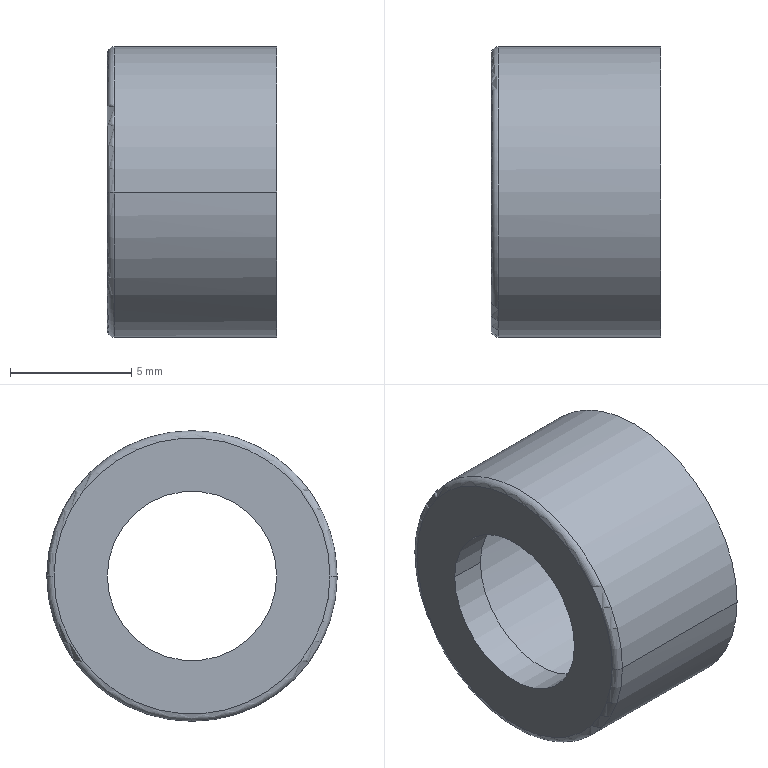Part | STEP file | SHIMOZHOUCHENGWAITAO_6_1_2_3_2_ | 1 solid | 15 faces | box 7 x 12 x 12 mm | volume 297.806 mm3 | cylinder 6 | torus 4 | plane 3 | cone 2 | commonest cylinder face diameters 7 x2 10 x2 12 x2
STEP:
#1=CARTESIAN_POINT('',(0.,0.,0.));
#2=DIRECTION('',(0.,0.,1.));
#3=DIRECTION('',(1.,0.,0.));
#4=AXIS2_PLACEMENT_3D('',#1,#2,#3);
#5=CARTESIAN_POINT('',(0.,-5.7,-0.03809));
#6=VERTEX_POINT('',#5);
#7=CARTESIAN_POINT('',(0.,-5.7,0.));
#8=VERTEX_POINT('',#7);
#9=CARTESIAN_POINT('',(0.,0.,0.));
#10=DIRECTION('',(-1.,0.,0.));
#11=DIRECTION('',(0.,-1.,-0.006683));
#12=AXIS2_PLACEMENT_3D('',#9,#10,#11);
#13=CIRCLE('',#12,5.7);
#14=EDGE_CURVE('',#6,#8,#13,.T.);
#15=ORIENTED_EDGE('',*,*,#14,.F.);
#16=CARTESIAN_POINT('',(0.,5.7,0.));
#17=VERTEX_POINT('',#16);
#18=CARTESIAN_POINT('',(0.,0.,0.));
#19=DIRECTION('',(1.,0.,0.));
#20=DIRECTION('',(0.,-1.,-0.006683));
#21=AXIS2_PLACEMENT_3D('',#18,#19,#20);
#22=CIRCLE('',#21,5.7);
#23=EDGE_CURVE('',#6,#17,#22,.T.);
#24=ORIENTED_EDGE('',*,*,#23,.T.);
#25=CARTESIAN_POINT('',(0.,5.7,0.03809));
#26=VERTEX_POINT('',#25);
#27=CARTESIAN_POINT('',(0.,0.,0.));
#28=DIRECTION('',(-1.,0.,0.));
#29=DIRECTION('',(0.,1.,0.006683));
#30=AXIS2_PLACEMENT_3D('',#27,#28,#29);
#31=CIRCLE('',#30,5.7);
#32=EDGE_CURVE('',#26,#17,#31,.T.);
#33=ORIENTED_EDGE('',*,*,#32,.F.);
#34=CARTESIAN_POINT('',(0.,0.,0.));
#35=DIRECTION('',(1.,0.,0.));
#36=DIRECTION('',(0.,1.,0.006683));
#37=AXIS2_PLACEMENT_3D('',#34,#35,#36);
#38=CIRCLE('',#37,5.7);
#39=EDGE_CURVE('',#26,#8,#38,.T.);
#40=ORIENTED_EDGE('',*,*,#39,.T.);
#41=EDGE_LOOP('',(#15,#24,#33,#40));
#42=FACE_OUTER_BOUND('',#41,.F.);
#43=CARTESIAN_POINT('',(0.,3.5,0.));
#44=VERTEX_POINT('',#43);
#45=CARTESIAN_POINT('',(0.,-3.5,0.));
#46=VERTEX_POINT('',#45);
#47=CARTESIAN_POINT('',(0.,0.,0.));
#48=DIRECTION('',(-1.,0.,0.));
#49=DIRECTION('',(0.,1.,0.));
#50=AXIS2_PLACEMENT_3D('',#47,#48,#49);
#51=CIRCLE('',#50,3.5);
#52=EDGE_CURVE('',#44,#46,#51,.T.);
#53=ORIENTED_EDGE('',*,*,#52,.T.);
#54=CARTESIAN_POINT('',(0.,0.,0.));
#55=DIRECTION('',(-1.,0.,0.));
#56=DIRECTION('',(0.,-1.,0.));
#57=AXIS2_PLACEMENT_3D('',#54,#55,#56);
#58=CIRCLE('',#57,3.5);
#59=EDGE_CURVE('',#46,#44,#58,.T.);
#60=ORIENTED_EDGE('',*,*,#59,.T.);
#61=EDGE_LOOP('',(#53,#60));
#62=FACE_BOUND('',#61,.F.);
#63=CARTESIAN_POINT('',(0.,0.,0.));
#64=DIRECTION('',(1.,0.,0.));
#65=DIRECTION('',(0.,-1.,0.));
#66=AXIS2_PLACEMENT_3D('',#63,#64,#65);
#67=PLANE('',#66);
#68=ADVANCED_FACE('',(#42,#62),#67,.F.);
#69=ORIENTED_EDGE('',*,*,#23,.F.);
#70=ORIENTED_EDGE('',*,*,#14,.T.);
#71=CARTESIAN_POINT('',(0.3,-6.,0.));
#72=VERTEX_POINT('',#71);
#73=CARTESIAN_POINT('',(0.3,-5.7,0.));
#74=DIRECTION('',(0.,0.,1.));
#75=DIRECTION('',(-1.,0.,0.));
#76=AXIS2_PLACEMENT_3D('',#73,#74,#75);
#77=CIRCLE('',#76,0.3);
#78=EDGE_CURVE('',#8,#72,#77,.T.);
#79=ORIENTED_EDGE('',*,*,#78,.T.);
#80=CARTESIAN_POINT('',(0.3,-6.,-0.0401));
#81=VERTEX_POINT('',#80);
#82=CARTESIAN_POINT('',(0.3,0.,0.));
#83=DIRECTION('',(1.,0.,0.));
#84=DIRECTION('',(0.,-1.,0.));
#85=AXIS2_PLACEMENT_3D('',#82,#83,#84);
#86=CIRCLE('',#85,6.);
#87=EDGE_CURVE('',#72,#81,#86,.T.);
#88=ORIENTED_EDGE('',*,*,#87,.T.);
#89=CARTESIAN_POINT('',(0.3,6.,0.));
#90=VERTEX_POINT('',#89);
#91=CARTESIAN_POINT('',(0.3,0.,0.));
#92=DIRECTION('',(1.,0.,0.));
#93=DIRECTION('',(0.,-1.,-0.006683));
#94=AXIS2_PLACEMENT_3D('',#91,#92,#93);
#95=CIRCLE('',#94,6.);
#96=EDGE_CURVE('',#81,#90,#95,.T.);
#97=ORIENTED_EDGE('',*,*,#96,.T.);
#98=CARTESIAN_POINT('',(0.3,5.7,0.));
#99=DIRECTION('',(0.,0.,-1.));
#100=DIRECTION('',(-1.,0.,0.));
#101=AXIS2_PLACEMENT_3D('',#98,#99,#100);
#102=CIRCLE('',#101,0.3);
#103=EDGE_CURVE('',#17,#90,#102,.T.);
#104=ORIENTED_EDGE('',*,*,#103,.F.);
#105=EDGE_LOOP('',(#69,#70,#79,#88,#97,#104));
#106=FACE_OUTER_BOUND('',#105,.F.);
#107=CARTESIAN_POINT('',(0.3,0.,0.));
#108=DIRECTION('',(1.,0.,0.));
#109=DIRECTION('',(0.,1.,0.006683));
#110=AXIS2_PLACEMENT_3D('',#107,#108,#109);
#111=TOROIDAL_SURFACE('',#110,5.7,0.3);
#112=ADVANCED_FACE('',(#106),#111,.T.);
#113=ORIENTED_EDGE('',*,*,#39,.F.);
#114=ORIENTED_EDGE('',*,*,#32,.T.);
#115=ORIENTED_EDGE('',*,*,#103,.T.);
#116=CARTESIAN_POINT('',(0.3,6.,0.0401));
#117=VERTEX_POINT('',#116);
#118=CARTESIAN_POINT('',(0.3,0.,0.));
#119=DIRECTION('',(1.,0.,0.));
#120=DIRECTION('',(0.,1.,0.));
#121=AXIS2_PLACEMENT_3D('',#118,#119,#120);
#122=CIRCLE('',#121,6.);
#123=EDGE_CURVE('',#90,#117,#122,.T.);
#124=ORIENTED_EDGE('',*,*,#123,.T.);
#125=CARTESIAN_POINT('',(0.3,0.,0.));
#126=DIRECTION('',(1.,0.,0.));
#127=DIRECTION('',(0.,1.,0.006683));
#128=AXIS2_PLACEMENT_3D('',#125,#126,#127);
#129=CIRCLE('',#128,6.);
#130=EDGE_CURVE('',#117,#72,#129,.T.);
#131=ORIENTED_EDGE('',*,*,#130,.T.);
#132=ORIENTED_EDGE('',*,*,#78,.F.);
#133=EDGE_LOOP('',(#113,#114,#115,#124,#131,#132));
#134=FACE_OUTER_BOUND('',#133,.F.);
#135=CARTESIAN_POINT('',(0.3,0.,0.));
#136=DIRECTION('',(1.,0.,0.));
#137=DIRECTION('',(0.,-1.,-0.006683));
#138=AXIS2_PLACEMENT_3D('',#135,#136,#137);
#139=TOROIDAL_SURFACE('',#138,5.7,0.3);
#140=ADVANCED_FACE('',(#134),#139,.T.);
#141=ORIENTED_EDGE('',*,*,#130,.F.);
#142=ORIENTED_EDGE('',*,*,#123,.F.);
#143=CARTESIAN_POINT('',(7.,6.,0.));
#144=VERTEX_POINT('',#143);
#145=CARTESIAN_POINT('',(0.3,6.,0.));
#146=DIRECTION('',(1.,0.,0.));
#147=VECTOR('',#146,6.7);
#148=LINE('',#145,#147);
#149=EDGE_CURVE('',#90,#144,#148,.T.);
#150=ORIENTED_EDGE('',*,*,#149,.T.);
#151=CARTESIAN_POINT('',(7.,-6.,0.));
#152=VERTEX_POINT('',#151);
#153=CARTESIAN_POINT('',(7.,0.,0.));
#154=DIRECTION('',(-1.,0.,0.));
#155=DIRECTION('',(0.,-1.,0.));
#156=AXIS2_PLACEMENT_3D('',#153,#154,#155);
#157=CIRCLE('',#156,6.);
#158=EDGE_CURVE('',#152,#144,#157,.T.);
#159=ORIENTED_EDGE('',*,*,#158,.F.);
#160=CARTESIAN_POINT('',(0.3,-6.,0.));
#161=DIRECTION('',(1.,0.,0.));
#162=VECTOR('',#161,6.7);
#163=LINE('',#160,#162);
#164=EDGE_CURVE('',#72,#152,#163,.T.);
#165=ORIENTED_EDGE('',*,*,#164,.F.);
#166=EDGE_LOOP('',(#141,#142,#150,#159,#165));
#167=FACE_OUTER_BOUND('',#166,.F.);
#168=CARTESIAN_POINT('',(0.,0.,0.));
#169=DIRECTION('',(1.,0.,0.));
#170=DIRECTION('',(0.,-1.,0.));
#171=AXIS2_PLACEMENT_3D('',#168,#169,#170);
#172=CYLINDRICAL_SURFACE('',#171,6.);
#173=ADVANCED_FACE('',(#167),#172,.T.);
#174=ORIENTED_EDGE('',*,*,#96,.F.);
#175=ORIENTED_EDGE('',*,*,#87,.F.);
#176=ORIENTED_EDGE('',*,*,#164,.T.);
#177=CARTESIAN_POINT('',(7.,0.,0.));
#178=DIRECTION('',(-1.,0.,0.));
#179=DIRECTION('',(0.,1.,0.));
#180=AXIS2_PLACEMENT_3D('',#177,#178,#179);
#181=CIRCLE('',#180,6.);
#182=EDGE_CURVE('',#144,#152,#181,.T.);
#183=ORIENTED_EDGE('',*,*,#182,.F.);
#184=ORIENTED_EDGE('',*,*,#149,.F.);
#185=EDGE_LOOP('',(#174,#175,#176,#183,#184));
#186=FACE_OUTER_BOUND('',#185,.F.);
#187=CARTESIAN_POINT('',(0.,0.,0.));
#188=DIRECTION('',(1.,0.,0.));
#189=DIRECTION('',(0.,-1.,0.));
#190=AXIS2_PLACEMENT_3D('',#187,#188,#189);
#191=CYLINDRICAL_SURFACE('',#190,6.);
#192=ADVANCED_FACE('',(#186),#191,.T.);
#193=ORIENTED_EDGE('',*,*,#182,.T.);
#194=ORIENTED_EDGE('',*,*,#158,.T.);
#195=EDGE_LOOP('',(#193,#194));
#196=FACE_OUTER_BOUND('',#195,.F.);
#197=CARTESIAN_POINT('',(7.,-5.5,0.));
#198=VERTEX_POINT('',#197);
#199=CARTESIAN_POINT('',(7.,0.,-5.5));
#200=VERTEX_POINT('',#199);
#201=CARTESIAN_POINT('',(7.,0.,0.));
#202=DIRECTION('',(1.,0.,0.));
#203=DIRECTION('',(0.,-1.,0.));
#204=AXIS2_PLACEMENT_3D('',#201,#202,#203);
#205=CIRCLE('',#204,5.5);
#206=EDGE_CURVE('',#198,#200,#205,.T.);
#207=ORIENTED_EDGE('',*,*,#206,.T.);
#208=CARTESIAN_POINT('',(7.,5.5,0.));
#209=VERTEX_POINT('',#208);
#210=CARTESIAN_POINT('',(7.,0.,0.));
#211=DIRECTION('',(1.,0.,0.));
#212=DIRECTION('',(0.,0.,-1.));
#213=AXIS2_PLACEMENT_3D('',#210,#211,#212);
#214=CIRCLE('',#213,5.5);
#215=EDGE_CURVE('',#200,#209,#214,.T.);
#216=ORIENTED_EDGE('',*,*,#215,.T.);
#217=CARTESIAN_POINT('',(7.,0.,5.5));
#218=VERTEX_POINT('',#217);
#219=CARTESIAN_POINT('',(7.,0.,0.));
#220=DIRECTION('',(1.,0.,0.));
#221=DIRECTION('',(0.,1.,0.));
#222=AXIS2_PLACEMENT_3D('',#219,#220,#221);
#223=CIRCLE('',#222,5.5);
#224=EDGE_CURVE('',#209,#218,#223,.T.);
#225=ORIENTED_EDGE('',*,*,#224,.T.);
#226=CARTESIAN_POINT('',(7.,0.,0.));
#227=DIRECTION('',(1.,0.,0.));
#228=DIRECTION('',(0.,0.,1.));
#229=AXIS2_PLACEMENT_3D('',#226,#227,#228);
#230=CIRCLE('',#229,5.5);
#231=EDGE_CURVE('',#218,#198,#230,.T.);
#232=ORIENTED_EDGE('',*,*,#231,.T.);
#233=EDGE_LOOP('',(#207,#216,#225,#232));
#234=FACE_BOUND('',#233,.F.);
#235=CARTESIAN_POINT('',(7.,0.,0.));
#236=DIRECTION('',(1.,0.,0.));
#237=DIRECTION('',(0.,-1.,0.));
#238=AXIS2_PLACEMENT_3D('',#235,#236,#237);
#239=PLANE('',#238);
#240=ADVANCED_FACE('',(#196,#234),#239,.T.);
#241=ORIENTED_EDGE('',*,*,#215,.F.);
#242=ORIENTED_EDGE('',*,*,#206,.F.);
#243=CARTESIAN_POINT('',(6.5,-5.,0.));
#244=VERTEX_POINT('',#243);
#245=CARTESIAN_POINT('',(7.,-5.5,0.));
#246=DIRECTION('',(-0.7071,0.7071,0.));
#247=VECTOR('',#246,0.7071);
#248=LINE('',#245,#247);
#249=EDGE_CURVE('',#198,#244,#248,.T.);
#250=ORIENTED_EDGE('',*,*,#249,.T.);
#251=CARTESIAN_POINT('',(6.5,0.,-5.));
#252=VERTEX_POINT('',#251);
#253=CARTESIAN_POINT('',(6.5,0.,0.));
#254=DIRECTION('',(1.,0.,0.));
#255=DIRECTION('',(0.,-1.,0.));
#256=AXIS2_PLACEMENT_3D('',#253,#254,#255);
#257=CIRCLE('',#256,5.);
#258=EDGE_CURVE('',#244,#252,#257,.T.);
#259=ORIENTED_EDGE('',*,*,#258,.T.);
#260=CARTESIAN_POINT('',(6.5,5.,0.));
#261=VERTEX_POINT('',#260);
#262=CARTESIAN_POINT('',(6.5,0.,0.));
#263=DIRECTION('',(1.,0.,0.));
#264=DIRECTION('',(0.,0.,-1.));
#265=AXIS2_PLACEMENT_3D('',#262,#263,#264);
#266=CIRCLE('',#265,5.);
#267=EDGE_CURVE('',#252,#261,#266,.T.);
#268=ORIENTED_EDGE('',*,*,#267,.T.);
#269=CARTESIAN_POINT('',(7.,5.5,0.));
#270=DIRECTION('',(-0.7071,-0.7071,0.));
#271=VECTOR('',#270,0.7071);
#272=LINE('',#269,#271);
#273=EDGE_CURVE('',#209,#261,#272,.T.);
#274=ORIENTED_EDGE('',*,*,#273,.F.);
#275=EDGE_LOOP('',(#241,#242,#250,#259,#268,#274));
#276=FACE_OUTER_BOUND('',#275,.F.);
#277=CARTESIAN_POINT('',(6.75,0.,0.));
#278=DIRECTION('',(1.,0.,0.));
#279=DIRECTION('',(0.,0.,-1.));
#280=AXIS2_PLACEMENT_3D('',#277,#278,#279);
#281=CONICAL_SURFACE('',#280,5.25,45.);
#282=ADVANCED_FACE('',(#276),#281,.F.);
#283=ORIENTED_EDGE('',*,*,#231,.F.);
#284=ORIENTED_EDGE('',*,*,#224,.F.);
#285=ORIENTED_EDGE('',*,*,#273,.T.);
#286=CARTESIAN_POINT('',(6.5,0.,5.));
#287=VERTEX_POINT('',#286);
#288=CARTESIAN_POINT('',(6.5,0.,0.));
#289=DIRECTION('',(1.,0.,0.));
#290=DIRECTION('',(0.,1.,0.));
#291=AXIS2_PLACEMENT_3D('',#288,#289,#290);
#292=CIRCLE('',#291,5.);
#293=EDGE_CURVE('',#261,#287,#292,.T.);
#294=ORIENTED_EDGE('',*,*,#293,.T.);
#295=CARTESIAN_POINT('',(6.5,0.,0.));
#296=DIRECTION('',(1.,0.,0.));
#297=DIRECTION('',(0.,0.,1.));
#298=AXIS2_PLACEMENT_3D('',#295,#296,#297);
#299=CIRCLE('',#298,5.);
#300=EDGE_CURVE('',#287,#244,#299,.T.);
#301=ORIENTED_EDGE('',*,*,#300,.T.);
#302=ORIENTED_EDGE('',*,*,#249,.F.);
#303=EDGE_LOOP('',(#283,#284,#285,#294,#301,#302));
#304=FACE_OUTER_BOUND('',#303,.F.);
#305=CARTESIAN_POINT('',(6.75,0.,0.));
#306=DIRECTION('',(1.,0.,0.));
#307=DIRECTION('',(0.,0.,-1.));
#308=AXIS2_PLACEMENT_3D('',#305,#306,#307);
#309=CONICAL_SURFACE('',#308,5.25,45.);
#310=ADVANCED_FACE('',(#304),#309,.F.);
#311=ORIENTED_EDGE('',*,*,#300,.F.);
#312=ORIENTED_EDGE('',*,*,#293,.F.);
#313=CARTESIAN_POINT('',(1.8,5.,0.));
#314=VERTEX_POINT('',#313);
#315=CARTESIAN_POINT('',(1.8,5.,0.));
#316=DIRECTION('',(1.,0.,0.));
#317=VECTOR('',#316,4.7);
#318=LINE('',#315,#317);
#319=EDGE_CURVE('',#314,#261,#318,.T.);
#320=ORIENTED_EDGE('',*,*,#319,.F.);
#321=CARTESIAN_POINT('',(1.8,-5.,0.02959));
#322=VERTEX_POINT('',#321);
#323=CARTESIAN_POINT('',(1.8,0.,0.));
#324=DIRECTION('',(-1.,0.,0.));
#325=DIRECTION('',(0.,-1.,0.005918));
#326=AXIS2_PLACEMENT_3D('',#323,#324,#325);
#327=CIRCLE('',#326,5.);
#328=EDGE_CURVE('',#322,#314,#327,.T.);
#329=ORIENTED_EDGE('',*,*,#328,.F.);
#330=CARTESIAN_POINT('',(1.8,-5.,0.));
#331=VERTEX_POINT('',#330);
#332=CARTESIAN_POINT('',(1.8,0.,0.));
#333=DIRECTION('',(-1.,0.,0.));
#334=DIRECTION('',(0.,-1.,0.));
#335=AXIS2_PLACEMENT_3D('',#332,#333,#334);
#336=CIRCLE('',#335,5.);
#337=EDGE_CURVE('',#331,#322,#336,.T.);
#338=ORIENTED_EDGE('',*,*,#337,.F.);
#339=CARTESIAN_POINT('',(1.8,-5.,0.));
#340=DIRECTION('',(1.,0.,0.));
#341=VECTOR('',#340,4.7);
#342=LINE('',#339,#341);
#343=EDGE_CURVE('',#331,#244,#342,.T.);
#344=ORIENTED_EDGE('',*,*,#343,.T.);
#345=EDGE_LOOP('',(#311,#312,#320,#329,#338,#344));
#346=FACE_OUTER_BOUND('',#345,.F.);
#347=CARTESIAN_POINT('',(0.,0.,0.));
#348=DIRECTION('',(1.,0.,0.));
#349=DIRECTION('',(0.,-1.,0.));
#350=AXIS2_PLACEMENT_3D('',#347,#348,#349);
#351=CYLINDRICAL_SURFACE('',#350,5.);
#352=ADVANCED_FACE('',(#346),#351,.F.);
#353=ORIENTED_EDGE('',*,*,#267,.F.);
#354=ORIENTED_EDGE('',*,*,#258,.F.);
#355=ORIENTED_EDGE('',*,*,#343,.F.);
#356=CARTESIAN_POINT('',(1.8,5.,-0.02959));
#357=VERTEX_POINT('',#356);
#358=CARTESIAN_POINT('',(1.8,0.,0.));
#359=DIRECTION('',(-1.,0.,0.));
#360=DIRECTION('',(0.,1.,-0.005918));
#361=AXIS2_PLACEMENT_3D('',#358,#359,#360);
#362=CIRCLE('',#361,5.);
#363=EDGE_CURVE('',#357,#331,#362,.T.);
#364=ORIENTED_EDGE('',*,*,#363,.F.);
#365=CARTESIAN_POINT('',(1.8,0.,0.));
#366=DIRECTION('',(-1.,0.,0.));
#367=DIRECTION('',(0.,1.,0.));
#368=AXIS2_PLACEMENT_3D('',#365,#366,#367);
#369=CIRCLE('',#368,5.);
#370=EDGE_CURVE('',#314,#357,#369,.T.);
#371=ORIENTED_EDGE('',*,*,#370,.F.);
#372=ORIENTED_EDGE('',*,*,#319,.T.);
#373=EDGE_LOOP('',(#353,#354,#355,#364,#371,#372));
#374=FACE_OUTER_BOUND('',#373,.F.);
#375=CARTESIAN_POINT('',(0.,0.,0.));
#376=DIRECTION('',(1.,0.,0.));
#377=DIRECTION('',(0.,-1.,0.));
#378=AXIS2_PLACEMENT_3D('',#375,#376,#377);
#379=CYLINDRICAL_SURFACE('',#378,5.);
#380=ADVANCED_FACE('',(#374),#379,.F.);
#381=ORIENTED_EDGE('',*,*,#370,.T.);
#382=ORIENTED_EDGE('',*,*,#363,.T.);
#383=CARTESIAN_POINT('',(1.5,-4.7,0.));
#384=VERTEX_POINT('',#383);
#385=CARTESIAN_POINT('',(1.8,-4.7,0.));
#386=DIRECTION('',(0.,0.,-1.));
#387=DIRECTION('',(0.,-1.,0.));
#388=AXIS2_PLACEMENT_3D('',#385,#386,#387);
#389=CIRCLE('',#388,0.3);
#390=EDGE_CURVE('',#331,#384,#389,.T.);
#391=ORIENTED_EDGE('',*,*,#390,.T.);
#392=CARTESIAN_POINT('',(1.5,4.7,-0.02781));
#393=VERTEX_POINT('',#392);
#394=CARTESIAN_POINT('',(1.5,0.,0.));
#395=DIRECTION('',(-1.,0.,0.));
#396=DIRECTION('',(0.,1.,-0.005917));
#397=AXIS2_PLACEMENT_3D('',#394,#395,#396);
#398=CIRCLE('',#397,4.7);
#399=EDGE_CURVE('',#393,#384,#398,.T.);
#400=ORIENTED_EDGE('',*,*,#399,.F.);
#401=CARTESIAN_POINT('',(1.5,4.7,0.));
#402=VERTEX_POINT('',#401);
#403=CARTESIAN_POINT('',(1.5,0.,0.));
#404=DIRECTION('',(1.,0.,0.));
#405=DIRECTION('',(0.,1.,-0.005917));
#406=AXIS2_PLACEMENT_3D('',#403,#404,#405);
#407=CIRCLE('',#406,4.7);
#408=EDGE_CURVE('',#393,#402,#407,.T.);
#409=ORIENTED_EDGE('',*,*,#408,.T.);
#410=CARTESIAN_POINT('',(1.8,4.7,0.));
#411=DIRECTION('',(0.,0.,1.));
#412=DIRECTION('',(0.,1.,0.));
#413=AXIS2_PLACEMENT_3D('',#410,#411,#412);
#414=CIRCLE('',#413,0.3);
#415=EDGE_CURVE('',#314,#402,#414,.T.);
#416=ORIENTED_EDGE('',*,*,#415,.F.);
#417=EDGE_LOOP('',(#381,#382,#391,#400,#409,#416));
#418=FACE_OUTER_BOUND('',#417,.F.);
#419=CARTESIAN_POINT('',(1.8,0.,0.));
#420=DIRECTION('',(1.,0.,0.));
#421=DIRECTION('',(0.,-1.,0.005918));
#422=AXIS2_PLACEMENT_3D('',#419,#420,#421);
#423=TOROIDAL_SURFACE('',#422,4.7,0.3);
#424=ADVANCED_FACE('',(#418),#423,.F.);
#425=ORIENTED_EDGE('',*,*,#337,.T.);
#426=ORIENTED_EDGE('',*,*,#328,.T.);
#427=ORIENTED_EDGE('',*,*,#415,.T.);
#428=CARTESIAN_POINT('',(1.5,-4.7,0.02781));
#429=VERTEX_POINT('',#428);
#430=CARTESIAN_POINT('',(1.5,0.,0.));
#431=DIRECTION('',(-1.,0.,0.));
#432=DIRECTION('',(0.,-1.,0.005917));
#433=AXIS2_PLACEMENT_3D('',#430,#431,#432);
#434=CIRCLE('',#433,4.7);
#435=EDGE_CURVE('',#429,#402,#434,.T.);
#436=ORIENTED_EDGE('',*,*,#435,.F.);
#437=CARTESIAN_POINT('',(1.5,0.,0.));
#438=DIRECTION('',(1.,0.,0.));
#439=DIRECTION('',(0.,-1.,0.005917));
#440=AXIS2_PLACEMENT_3D('',#437,#438,#439);
#441=CIRCLE('',#440,4.7);
#442=EDGE_CURVE('',#429,#384,#441,.T.);
#443=ORIENTED_EDGE('',*,*,#442,.T.);
#444=ORIENTED_EDGE('',*,*,#390,.F.);
#445=EDGE_LOOP('',(#425,#426,#427,#436,#443,#444));
#446=FACE_OUTER_BOUND('',#445,.F.);
#447=CARTESIAN_POINT('',(1.8,0.,0.));
#448=DIRECTION('',(1.,0.,0.));
#449=DIRECTION('',(0.,1.,-0.005918));
#450=AXIS2_PLACEMENT_3D('',#447,#448,#449);
#451=TOROIDAL_SURFACE('',#450,4.7,0.3);
#452=ADVANCED_FACE('',(#446),#451,.F.);
#453=ORIENTED_EDGE('',*,*,#408,.F.);
#454=ORIENTED_EDGE('',*,*,#399,.T.);
#455=ORIENTED_EDGE('',*,*,#442,.F.);
#456=ORIENTED_EDGE('',*,*,#435,.T.);
#457=EDGE_LOOP('',(#453,#454,#455,#456));
#458=FACE_OUTER_BOUND('',#457,.F.);
#459=CARTESIAN_POINT('',(1.5,-3.5,0.));
#460=VERTEX_POINT('',#459);
#461=CARTESIAN_POINT('',(1.5,3.5,0.));
#462=VERTEX_POINT('',#461);
#463=CARTESIAN_POINT('',(1.5,0.,0.));
#464=DIRECTION('',(1.,0.,0.));
#465=DIRECTION('',(0.,-1.,0.));
#466=AXIS2_PLACEMENT_3D('',#463,#464,#465);
#467=CIRCLE('',#466,3.5);
#468=EDGE_CURVE('',#460,#462,#467,.T.);
#469=ORIENTED_EDGE('',*,*,#468,.T.);
#470=CARTESIAN_POINT('',(1.5,0.,0.));
#471=DIRECTION('',(1.,0.,0.));
#472=DIRECTION('',(0.,1.,0.));
#473=AXIS2_PLACEMENT_3D('',#470,#471,#472);
#474=CIRCLE('',#473,3.5);
#475=EDGE_CURVE('',#462,#460,#474,.T.);
#476=ORIENTED_EDGE('',*,*,#475,.T.);
#477=EDGE_LOOP('',(#469,#476));
#478=FACE_BOUND('',#477,.F.);
#479=CARTESIAN_POINT('',(1.5,0.,0.));
#480=DIRECTION('',(-1.,0.,0.));
#481=DIRECTION('',(0.,0.,-1.));
#482=AXIS2_PLACEMENT_3D('',#479,#480,#481);
#483=PLANE('',#482);
#484=ADVANCED_FACE('',(#458,#478),#483,.F.);
#485=ORIENTED_EDGE('',*,*,#52,.F.);
#486=CARTESIAN_POINT('',(1.5,3.5,0.));
#487=DIRECTION('',(-1.,0.,0.));
#488=VECTOR('',#487,1.5);
#489=LINE('',#486,#488);
#490=EDGE_CURVE('',#462,#44,#489,.T.);
#491=ORIENTED_EDGE('',*,*,#490,.F.);
#492=ORIENTED_EDGE('',*,*,#468,.F.);
#493=CARTESIAN_POINT('',(1.5,-3.5,0.));
#494=DIRECTION('',(-1.,0.,0.));
#495=VECTOR('',#494,1.5);
#496=LINE('',#493,#495);
#497=EDGE_CURVE('',#460,#46,#496,.T.);
#498=ORIENTED_EDGE('',*,*,#497,.T.);
#499=EDGE_LOOP('',(#485,#491,#492,#498));
#500=FACE_OUTER_BOUND('',#499,.F.);
#501=CARTESIAN_POINT('',(1.5,0.,0.));
#502=DIRECTION('',(1.,0.,0.));
#503=DIRECTION('',(0.,-1.,0.));
#504=AXIS2_PLACEMENT_3D('',#501,#502,#503);
#505=CYLINDRICAL_SURFACE('',#504,3.5);
#506=ADVANCED_FACE('',(#500),#505,.F.);
#507=ORIENTED_EDGE('',*,*,#59,.F.);
#508=ORIENTED_EDGE('',*,*,#497,.F.);
#509=ORIENTED_EDGE('',*,*,#475,.F.);
#510=ORIENTED_EDGE('',*,*,#490,.T.);
#511=EDGE_LOOP('',(#507,#508,#509,#510));
#512=FACE_OUTER_BOUND('',#511,.F.);
#513=CARTESIAN_POINT('',(1.5,0.,0.));
#514=DIRECTION('',(1.,0.,0.));
#515=DIRECTION('',(0.,-1.,0.));
#516=AXIS2_PLACEMENT_3D('',#513,#514,#515);
#517=CYLINDRICAL_SURFACE('',#516,3.5);
#518=ADVANCED_FACE('',(#512),#517,.F.);
#519=CLOSED_SHELL('',(#68,#112,#140,#173,#192,#240,#282,#310,#352,#380,#424,#452,#484,#506,#518));
#520=MANIFOLD_SOLID_BREP('',#519);
#521=(LENGTH_UNIT()NAMED_UNIT(*)SI_UNIT(.MILLI.,.METRE.));
#522=UNCERTAINTY_MEASURE_WITH_UNIT(LENGTH_MEASURE(0.001836),#521,'','');
#523=(NAMED_UNIT(*)PLANE_ANGLE_UNIT()SI_UNIT($,.RADIAN.));
#524=PLANE_ANGLE_MEASURE_WITH_UNIT(PLANE_ANGLE_MEASURE(0.01745),#523);
#525=(CONVERSION_BASED_UNIT('DEGREE',#524)NAMED_UNIT(*)PLANE_ANGLE_UNIT());
#526=(NAMED_UNIT(*)SI_UNIT($,.STERADIAN.)SOLID_ANGLE_UNIT());
#527=(GEOMETRIC_REPRESENTATION_CONTEXT(3)GLOBAL_UNCERTAINTY_ASSIGNED_CONTEXT((#522))GLOBAL_UNIT_ASSIGNED_CONTEXT((#521,#525,#526))REPRESENTATION_CONTEXT('',''));
#528=ADVANCED_BREP_SHAPE_REPRESENTATION('',(#4,#520),#527);